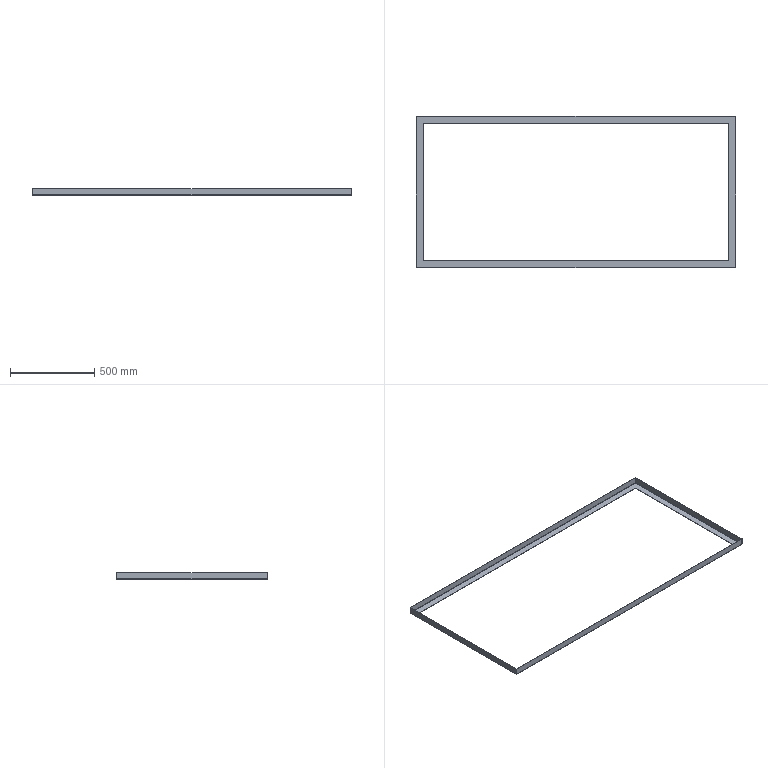Part | SolidWorks | features EdgeFlange 1, FlatPattern 1, ICE 1, SMBaseFlange 1, SheetMetal 1 | 1 solid | 42 faces | box 1900 x 900 x 40 mm | volume 850779 mm3 | plane 26 | spline 8 | cylinder 8 | commonest cylinder face diameters 1.473 x4 5.473 x4